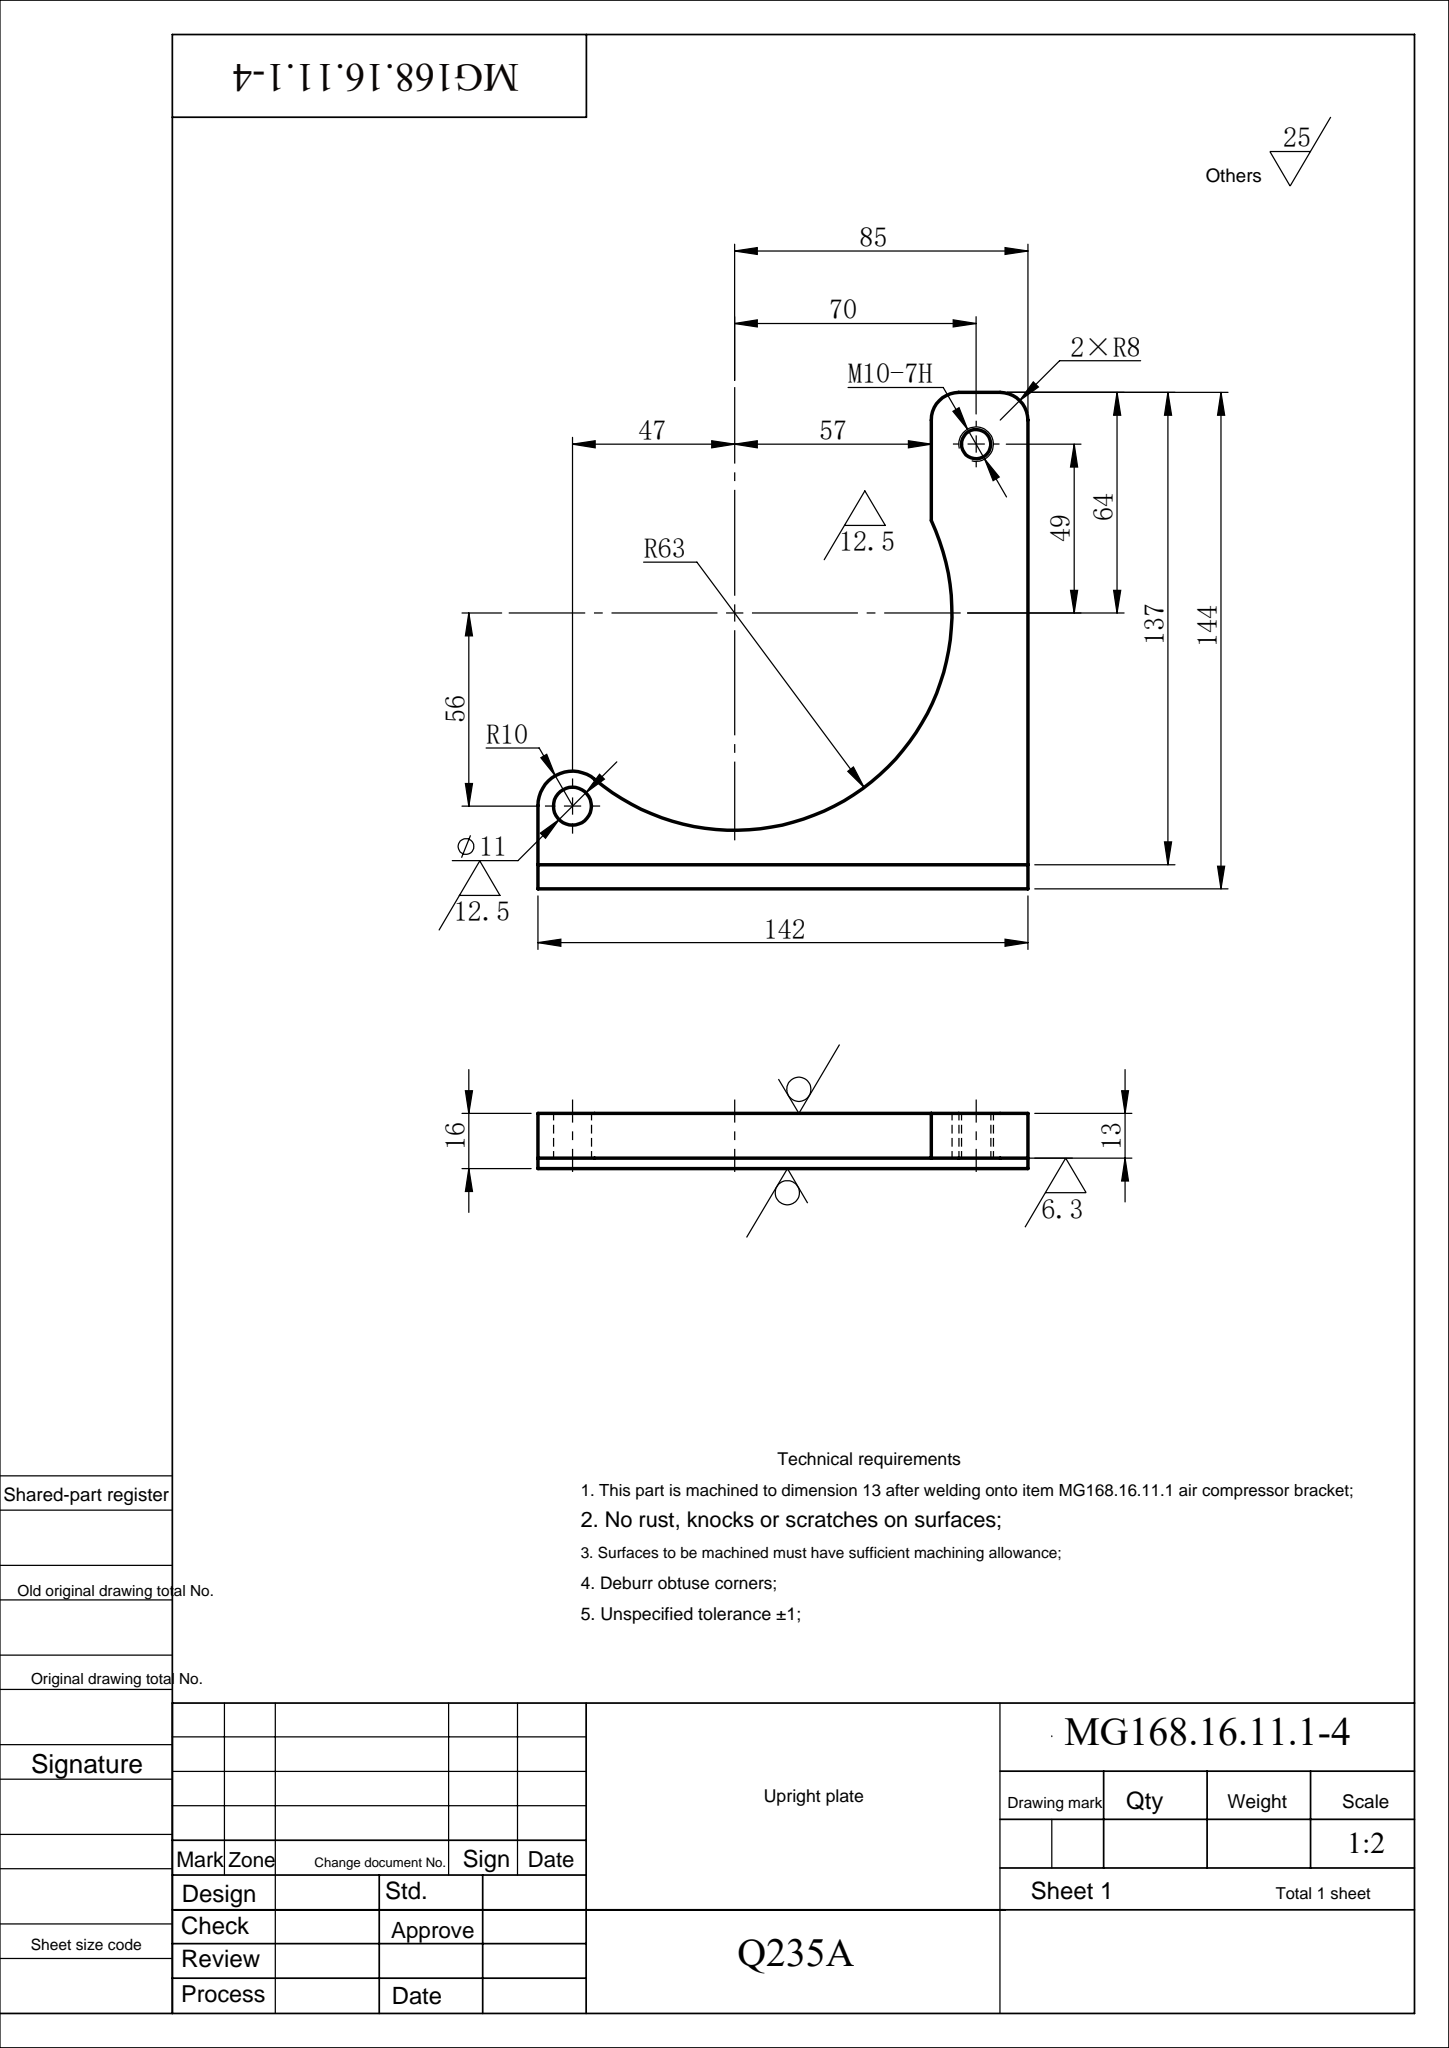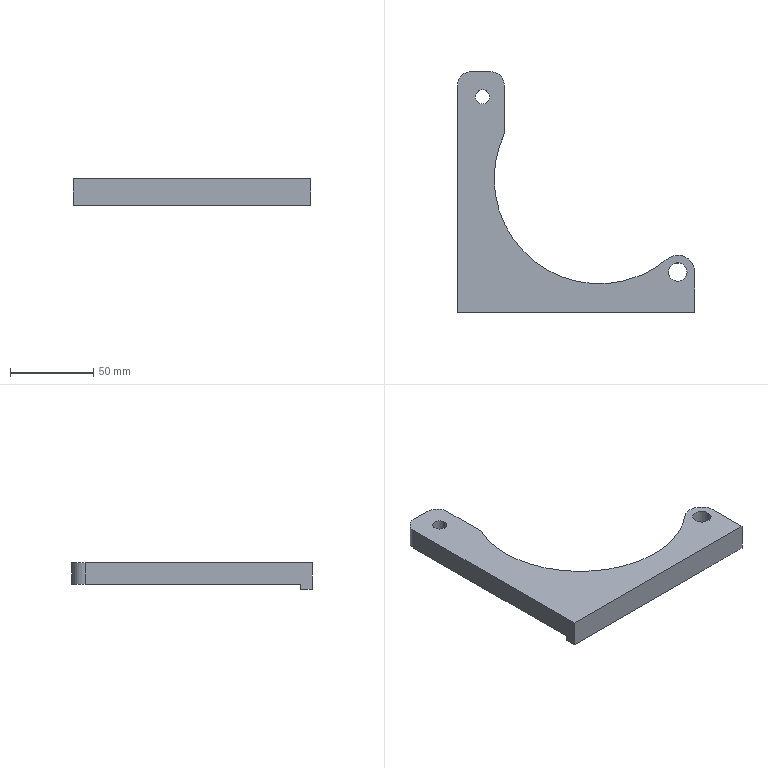Part | SolidWorks | features Extrusion 1, Fillet 1, HoleWzd 1, ICE 1 | 1 solid | 18 faces | box 142 x 144 x 16 mm | volume 88798 mm3 | cylinder 9 | plane 9 | commonest cylinder face diameters 8.5 x2 11 x2 16 x2 126 x2 20 x1
STEP:
#1=CARTESIAN_POINT('',(10.75,129.,-6.5));
#2=VERTEX_POINT('',#1);
#3=CARTESIAN_POINT('',(19.25,129.,-6.5));
#4=VERTEX_POINT('',#3);
#5=CARTESIAN_POINT('',(15.,129.,-6.5));
#6=DIRECTION('',(0.,0.,1.));
#7=DIRECTION('',(1.,0.,0.));
#8=AXIS2_PLACEMENT_3D('',#5,#6,#7);
#9=CIRCLE('',#8,4.25);
#10=EDGE_CURVE('',#2,#4,#9,.T.);
#11=ORIENTED_EDGE('',*,*,#10,.F.);
#12=CARTESIAN_POINT('',(10.75,129.,6.5));
#13=VERTEX_POINT('',#12);
#14=CARTESIAN_POINT('',(10.75,129.,6.5));
#15=DIRECTION('',(0.,0.,1.));
#16=VECTOR('',#15,1000.);
#17=LINE('',#14,#16);
#18=EDGE_CURVE('',#2,#13,#17,.T.);
#19=ORIENTED_EDGE('',*,*,#18,.T.);
#20=CARTESIAN_POINT('',(19.25,129.,6.5));
#21=VERTEX_POINT('',#20);
#22=CARTESIAN_POINT('',(15.,129.,6.5));
#23=DIRECTION('',(0.,0.,1.));
#24=DIRECTION('',(1.,0.,0.));
#25=AXIS2_PLACEMENT_3D('',#22,#23,#24);
#26=CIRCLE('',#25,4.25);
#27=EDGE_CURVE('',#13,#21,#26,.T.);
#28=ORIENTED_EDGE('',*,*,#27,.T.);
#29=CARTESIAN_POINT('',(19.25,129.,6.5));
#30=DIRECTION('',(0.,0.,1.));
#31=VECTOR('',#30,1000.);
#32=LINE('',#29,#31);
#33=EDGE_CURVE('',#4,#21,#32,.T.);
#34=ORIENTED_EDGE('',*,*,#33,.F.);
#35=EDGE_LOOP('',(#11,#19,#28,#34));
#36=FACE_OUTER_BOUND('',#35,.T.);
#37=CARTESIAN_POINT('',(15.,129.,6.5));
#38=DIRECTION('',(0.,0.,1.));
#39=DIRECTION('',(1.,0.,0.));
#40=AXIS2_PLACEMENT_3D('',#37,#38,#39);
#41=CYLINDRICAL_SURFACE('',#40,4.25);
#42=ADVANCED_FACE('',(#36),#41,.F.);
#43=CARTESIAN_POINT('',(126.5,24.,6.5));
#44=VERTEX_POINT('',#43);
#45=CARTESIAN_POINT('',(137.5,24.,6.5));
#46=VERTEX_POINT('',#45);
#47=CARTESIAN_POINT('',(132.,24.,6.5));
#48=DIRECTION('',(0.,0.,1.));
#49=DIRECTION('',(1.,0.,0.));
#50=AXIS2_PLACEMENT_3D('',#47,#48,#49);
#51=CIRCLE('',#50,5.5);
#52=EDGE_CURVE('',#44,#46,#51,.T.);
#53=ORIENTED_EDGE('',*,*,#52,.T.);
#54=CARTESIAN_POINT('',(137.5,24.,-6.5));
#55=VERTEX_POINT('',#54);
#56=CARTESIAN_POINT('',(137.5,24.,6.5));
#57=DIRECTION('',(0.,0.,-1.));
#58=VECTOR('',#57,1000.);
#59=LINE('',#56,#58);
#60=EDGE_CURVE('',#46,#55,#59,.T.);
#61=ORIENTED_EDGE('',*,*,#60,.T.);
#62=CARTESIAN_POINT('',(126.5,24.,-6.5));
#63=VERTEX_POINT('',#62);
#64=CARTESIAN_POINT('',(132.,24.,-6.5));
#65=DIRECTION('',(0.,0.,1.));
#66=DIRECTION('',(1.,0.,0.));
#67=AXIS2_PLACEMENT_3D('',#64,#65,#66);
#68=CIRCLE('',#67,5.5);
#69=EDGE_CURVE('',#63,#55,#68,.T.);
#70=ORIENTED_EDGE('',*,*,#69,.F.);
#71=CARTESIAN_POINT('',(126.5,24.,6.5));
#72=DIRECTION('',(0.,0.,-1.));
#73=VECTOR('',#72,1000.);
#74=LINE('',#71,#73);
#75=EDGE_CURVE('',#44,#63,#74,.T.);
#76=ORIENTED_EDGE('',*,*,#75,.F.);
#77=EDGE_LOOP('',(#53,#61,#70,#76));
#78=FACE_OUTER_BOUND('',#77,.T.);
#79=CARTESIAN_POINT('',(132.,24.,6.5));
#80=DIRECTION('',(0.,0.,-1.));
#81=DIRECTION('',(-1.,0.,0.));
#82=AXIS2_PLACEMENT_3D('',#79,#80,#81);
#83=CYLINDRICAL_SURFACE('',#82,5.5);
#84=ADVANCED_FACE('',(#78),#83,.F.);
#85=CARTESIAN_POINT('',(22.,80.,6.5));
#86=VERTEX_POINT('',#85);
#87=CARTESIAN_POINT('',(28.,106.833,6.5));
#88=VERTEX_POINT('',#87);
#89=CARTESIAN_POINT('',(85.,80.,6.5));
#90=DIRECTION('',(0.,0.,-1.));
#91=DIRECTION('',(1.,0.,0.));
#92=AXIS2_PLACEMENT_3D('',#89,#90,#91);
#93=CIRCLE('',#92,63.);
#94=EDGE_CURVE('',#86,#88,#93,.T.);
#95=ORIENTED_EDGE('',*,*,#94,.F.);
#96=CARTESIAN_POINT('',(22.,80.,-6.5));
#97=VERTEX_POINT('',#96);
#98=CARTESIAN_POINT('',(22.,80.,6.5));
#99=DIRECTION('',(0.,0.,-1.));
#100=VECTOR('',#99,1000.);
#101=LINE('',#98,#100);
#102=EDGE_CURVE('',#86,#97,#101,.T.);
#103=ORIENTED_EDGE('',*,*,#102,.T.);
#104=CARTESIAN_POINT('',(28.,106.833,-6.5));
#105=VERTEX_POINT('',#104);
#106=CARTESIAN_POINT('',(85.,80.,-6.5));
#107=DIRECTION('',(0.,0.,-1.));
#108=DIRECTION('',(1.,0.,0.));
#109=AXIS2_PLACEMENT_3D('',#106,#107,#108);
#110=CIRCLE('',#109,63.);
#111=EDGE_CURVE('',#97,#105,#110,.T.);
#112=ORIENTED_EDGE('',*,*,#111,.T.);
#113=CARTESIAN_POINT('',(28.,106.833,6.5));
#114=DIRECTION('',(0.,0.,-1.));
#115=VECTOR('',#114,1000.);
#116=LINE('',#113,#115);
#117=EDGE_CURVE('',#88,#105,#116,.T.);
#118=ORIENTED_EDGE('',*,*,#117,.F.);
#119=EDGE_LOOP('',(#95,#103,#112,#118));
#120=FACE_OUTER_BOUND('',#119,.T.);
#121=CARTESIAN_POINT('',(85.,80.,6.5));
#122=DIRECTION('',(0.,0.,-1.));
#123=DIRECTION('',(-1.,0.,0.));
#124=AXIS2_PLACEMENT_3D('',#121,#122,#123);
#125=CYLINDRICAL_SURFACE('',#124,63.);
#126=ADVANCED_FACE('',(#120),#125,.F.);
#127=CARTESIAN_POINT('',(15.,129.,6.5));
#128=DIRECTION('',(0.,0.,1.));
#129=DIRECTION('',(1.,0.,0.));
#130=AXIS2_PLACEMENT_3D('',#127,#128,#129);
#131=CIRCLE('',#130,4.25);
#132=EDGE_CURVE('',#21,#13,#131,.T.);
#133=ORIENTED_EDGE('',*,*,#132,.F.);
#134=ORIENTED_EDGE('',*,*,#27,.F.);
#135=EDGE_LOOP('',(#133,#134));
#136=FACE_BOUND('',#135,.T.);
#137=CARTESIAN_POINT('',(20.,144.,6.5));
#138=VERTEX_POINT('',#137);
#139=CARTESIAN_POINT('',(8.,144.,6.5));
#140=VERTEX_POINT('',#139);
#141=CARTESIAN_POINT('',(0.,144.,6.5));
#142=DIRECTION('',(-1.,0.,0.));
#143=VECTOR('',#142,1000.);
#144=LINE('',#141,#143);
#145=EDGE_CURVE('',#138,#140,#144,.T.);
#146=ORIENTED_EDGE('',*,*,#145,.T.);
#147=CARTESIAN_POINT('',(0.,136.,6.5));
#148=VERTEX_POINT('',#147);
#149=CARTESIAN_POINT('',(8.,136.,6.5));
#150=DIRECTION('',(0.,0.,1.));
#151=DIRECTION('',(1.,0.,0.));
#152=AXIS2_PLACEMENT_3D('',#149,#150,#151);
#153=CIRCLE('',#152,8.);
#154=EDGE_CURVE('',#140,#148,#153,.T.);
#155=ORIENTED_EDGE('',*,*,#154,.T.);
#156=CARTESIAN_POINT('',(0.,0.,6.5));
#157=VERTEX_POINT('',#156);
#158=CARTESIAN_POINT('',(0.,0.,6.5));
#159=DIRECTION('',(0.,-1.,0.));
#160=VECTOR('',#159,1000.);
#161=LINE('',#158,#160);
#162=EDGE_CURVE('',#148,#157,#161,.T.);
#163=ORIENTED_EDGE('',*,*,#162,.T.);
#164=CARTESIAN_POINT('',(142.,0.,6.5));
#165=VERTEX_POINT('',#164);
#166=CARTESIAN_POINT('',(0.,0.,6.5));
#167=DIRECTION('',(1.,0.,0.));
#168=VECTOR('',#167,1000.);
#169=LINE('',#166,#168);
#170=EDGE_CURVE('',#157,#165,#169,.T.);
#171=ORIENTED_EDGE('',*,*,#170,.T.);
#172=CARTESIAN_POINT('',(142.,24.143,6.5));
#173=VERTEX_POINT('',#172);
#174=CARTESIAN_POINT('',(142.,0.,6.5));
#175=DIRECTION('',(0.,1.,0.));
#176=VECTOR('',#175,1000.);
#177=LINE('',#174,#176);
#178=EDGE_CURVE('',#165,#173,#177,.T.);
#179=ORIENTED_EDGE('',*,*,#178,.T.);
#180=CARTESIAN_POINT('',(125.562,31.795,6.5));
#181=VERTEX_POINT('',#180);
#182=CARTESIAN_POINT('',(132.,24.143,6.5));
#183=DIRECTION('',(0.,0.,1.));
#184=DIRECTION('',(1.,0.,0.));
#185=AXIS2_PLACEMENT_3D('',#182,#183,#184);
#186=CIRCLE('',#185,10.);
#187=EDGE_CURVE('',#173,#181,#186,.T.);
#188=ORIENTED_EDGE('',*,*,#187,.T.);
#189=CARTESIAN_POINT('',(85.,80.,6.5));
#190=DIRECTION('',(0.,0.,-1.));
#191=DIRECTION('',(1.,0.,0.));
#192=AXIS2_PLACEMENT_3D('',#189,#190,#191);
#193=CIRCLE('',#192,63.);
#194=EDGE_CURVE('',#181,#86,#193,.T.);
#195=ORIENTED_EDGE('',*,*,#194,.T.);
#196=ORIENTED_EDGE('',*,*,#94,.T.);
#197=CARTESIAN_POINT('',(28.,136.,6.5));
#198=VERTEX_POINT('',#197);
#199=CARTESIAN_POINT('',(28.,144.,6.5));
#200=DIRECTION('',(0.,1.,0.));
#201=VECTOR('',#200,1000.);
#202=LINE('',#199,#201);
#203=EDGE_CURVE('',#88,#198,#202,.T.);
#204=ORIENTED_EDGE('',*,*,#203,.T.);
#205=CARTESIAN_POINT('',(20.,136.,6.5));
#206=DIRECTION('',(0.,0.,1.));
#207=DIRECTION('',(1.,0.,0.));
#208=AXIS2_PLACEMENT_3D('',#205,#206,#207);
#209=CIRCLE('',#208,8.);
#210=EDGE_CURVE('',#198,#138,#209,.T.);
#211=ORIENTED_EDGE('',*,*,#210,.T.);
#212=EDGE_LOOP('',(#146,#155,#163,#171,#179,#188,#195,#196,#204,#211));
#213=FACE_OUTER_BOUND('',#212,.T.);
#214=ORIENTED_EDGE('',*,*,#52,.F.);
#215=CARTESIAN_POINT('',(132.,24.,6.5));
#216=DIRECTION('',(0.,0.,1.));
#217=DIRECTION('',(1.,0.,0.));
#218=AXIS2_PLACEMENT_3D('',#215,#216,#217);
#219=CIRCLE('',#218,5.5);
#220=EDGE_CURVE('',#46,#44,#219,.T.);
#221=ORIENTED_EDGE('',*,*,#220,.F.);
#222=EDGE_LOOP('',(#214,#221));
#223=FACE_BOUND('',#222,.T.);
#224=CARTESIAN_POINT('',(85.,80.,6.5));
#225=DIRECTION('',(0.,0.,1.));
#226=DIRECTION('',(1.,0.,0.));
#227=AXIS2_PLACEMENT_3D('',#224,#225,#226);
#228=PLANE('',#227);
#229=ADVANCED_FACE('',(#136,#213,#223),#228,.T.);
#230=CARTESIAN_POINT('',(15.,129.,-6.5));
#231=DIRECTION('',(0.,0.,1.));
#232=DIRECTION('',(1.,0.,0.));
#233=AXIS2_PLACEMENT_3D('',#230,#231,#232);
#234=CIRCLE('',#233,4.25);
#235=EDGE_CURVE('',#4,#2,#234,.T.);
#236=ORIENTED_EDGE('',*,*,#235,.T.);
#237=ORIENTED_EDGE('',*,*,#10,.T.);
#238=EDGE_LOOP('',(#236,#237));
#239=FACE_BOUND('',#238,.T.);
#240=CARTESIAN_POINT('',(0.,136.,-6.5));
#241=VERTEX_POINT('',#240);
#242=CARTESIAN_POINT('',(0.,7.,-6.5));
#243=VERTEX_POINT('',#242);
#244=CARTESIAN_POINT('',(0.,0.,-6.5));
#245=DIRECTION('',(0.,-1.,0.));
#246=VECTOR('',#245,1000.);
#247=LINE('',#244,#246);
#248=EDGE_CURVE('',#241,#243,#247,.T.);
#249=ORIENTED_EDGE('',*,*,#248,.F.);
#250=CARTESIAN_POINT('',(8.,144.,-6.5));
#251=VERTEX_POINT('',#250);
#252=CARTESIAN_POINT('',(8.,136.,-6.5));
#253=DIRECTION('',(0.,0.,-1.));
#254=DIRECTION('',(1.,0.,0.));
#255=AXIS2_PLACEMENT_3D('',#252,#253,#254);
#256=CIRCLE('',#255,8.);
#257=EDGE_CURVE('',#241,#251,#256,.T.);
#258=ORIENTED_EDGE('',*,*,#257,.T.);
#259=CARTESIAN_POINT('',(20.,144.,-6.5));
#260=VERTEX_POINT('',#259);
#261=CARTESIAN_POINT('',(0.,144.,-6.5));
#262=DIRECTION('',(-1.,0.,0.));
#263=VECTOR('',#262,1000.);
#264=LINE('',#261,#263);
#265=EDGE_CURVE('',#260,#251,#264,.T.);
#266=ORIENTED_EDGE('',*,*,#265,.F.);
#267=CARTESIAN_POINT('',(28.,136.,-6.5));
#268=VERTEX_POINT('',#267);
#269=CARTESIAN_POINT('',(20.,136.,-6.5));
#270=DIRECTION('',(0.,0.,-1.));
#271=DIRECTION('',(1.,0.,0.));
#272=AXIS2_PLACEMENT_3D('',#269,#270,#271);
#273=CIRCLE('',#272,8.);
#274=EDGE_CURVE('',#260,#268,#273,.T.);
#275=ORIENTED_EDGE('',*,*,#274,.T.);
#276=CARTESIAN_POINT('',(28.,144.,-6.5));
#277=DIRECTION('',(0.,1.,0.));
#278=VECTOR('',#277,1000.);
#279=LINE('',#276,#278);
#280=EDGE_CURVE('',#105,#268,#279,.T.);
#281=ORIENTED_EDGE('',*,*,#280,.F.);
#282=ORIENTED_EDGE('',*,*,#111,.F.);
#283=CARTESIAN_POINT('',(125.562,31.795,-6.5));
#284=VERTEX_POINT('',#283);
#285=CARTESIAN_POINT('',(85.,80.,-6.5));
#286=DIRECTION('',(0.,0.,-1.));
#287=DIRECTION('',(1.,0.,0.));
#288=AXIS2_PLACEMENT_3D('',#285,#286,#287);
#289=CIRCLE('',#288,63.);
#290=EDGE_CURVE('',#284,#97,#289,.T.);
#291=ORIENTED_EDGE('',*,*,#290,.F.);
#292=CARTESIAN_POINT('',(142.,24.143,-6.5));
#293=VERTEX_POINT('',#292);
#294=CARTESIAN_POINT('',(132.,24.143,-6.5));
#295=DIRECTION('',(0.,0.,1.));
#296=DIRECTION('',(1.,0.,0.));
#297=AXIS2_PLACEMENT_3D('',#294,#295,#296);
#298=CIRCLE('',#297,10.);
#299=EDGE_CURVE('',#293,#284,#298,.T.);
#300=ORIENTED_EDGE('',*,*,#299,.F.);
#301=CARTESIAN_POINT('',(142.,7.,-6.5));
#302=VERTEX_POINT('',#301);
#303=CARTESIAN_POINT('',(142.,0.,-6.5));
#304=DIRECTION('',(0.,1.,0.));
#305=VECTOR('',#304,1000.);
#306=LINE('',#303,#305);
#307=EDGE_CURVE('',#302,#293,#306,.T.);
#308=ORIENTED_EDGE('',*,*,#307,.F.);
#309=CARTESIAN_POINT('',(0.,7.,-6.5));
#310=DIRECTION('',(-1.,0.,0.));
#311=VECTOR('',#310,1000.);
#312=LINE('',#309,#311);
#313=EDGE_CURVE('',#302,#243,#312,.T.);
#314=ORIENTED_EDGE('',*,*,#313,.T.);
#315=EDGE_LOOP('',(#249,#258,#266,#275,#281,#282,#291,#300,#308,#314));
#316=FACE_OUTER_BOUND('',#315,.T.);
#317=ORIENTED_EDGE('',*,*,#69,.T.);
#318=CARTESIAN_POINT('',(132.,24.,-6.5));
#319=DIRECTION('',(0.,0.,1.));
#320=DIRECTION('',(1.,0.,0.));
#321=AXIS2_PLACEMENT_3D('',#318,#319,#320);
#322=CIRCLE('',#321,5.5);
#323=EDGE_CURVE('',#55,#63,#322,.T.);
#324=ORIENTED_EDGE('',*,*,#323,.T.);
#325=EDGE_LOOP('',(#317,#324));
#326=FACE_BOUND('',#325,.T.);
#327=CARTESIAN_POINT('',(85.,80.,-6.5));
#328=DIRECTION('',(0.,0.,1.));
#329=DIRECTION('',(1.,0.,0.));
#330=AXIS2_PLACEMENT_3D('',#327,#328,#329);
#331=PLANE('',#330);
#332=ADVANCED_FACE('',(#239,#316,#326),#331,.F.);
#333=ORIENTED_EDGE('',*,*,#162,.F.);
#334=CARTESIAN_POINT('',(0.,136.,6.5));
#335=DIRECTION('',(0.,0.,-1.));
#336=VECTOR('',#335,1000.);
#337=LINE('',#334,#336);
#338=EDGE_CURVE('',#148,#241,#337,.T.);
#339=ORIENTED_EDGE('',*,*,#338,.T.);
#340=ORIENTED_EDGE('',*,*,#248,.T.);
#341=CARTESIAN_POINT('',(0.,7.,-9.5));
#342=VERTEX_POINT('',#341);
#343=CARTESIAN_POINT('',(0.,7.,-9.5));
#344=DIRECTION('',(0.,0.,1.));
#345=VECTOR('',#344,1000.);
#346=LINE('',#343,#345);
#347=EDGE_CURVE('',#342,#243,#346,.T.);
#348=ORIENTED_EDGE('',*,*,#347,.F.);
#349=CARTESIAN_POINT('',(0.,0.,-9.5));
#350=VERTEX_POINT('',#349);
#351=CARTESIAN_POINT('',(0.,0.,-9.5));
#352=DIRECTION('',(0.,-1.,0.));
#353=VECTOR('',#352,1000.);
#354=LINE('',#351,#353);
#355=EDGE_CURVE('',#342,#350,#354,.T.);
#356=ORIENTED_EDGE('',*,*,#355,.T.);
#357=CARTESIAN_POINT('',(0.,0.,6.5));
#358=DIRECTION('',(0.,0.,-1.));
#359=VECTOR('',#358,1000.);
#360=LINE('',#357,#359);
#361=EDGE_CURVE('',#157,#350,#360,.T.);
#362=ORIENTED_EDGE('',*,*,#361,.F.);
#363=EDGE_LOOP('',(#333,#339,#340,#348,#356,#362));
#364=FACE_OUTER_BOUND('',#363,.T.);
#365=CARTESIAN_POINT('',(0.,0.,6.5));
#366=DIRECTION('',(1.,0.,0.));
#367=DIRECTION('',(0.,0.,-1.));
#368=AXIS2_PLACEMENT_3D('',#365,#366,#367);
#369=PLANE('',#368);
#370=ADVANCED_FACE('',(#364),#369,.F.);
#371=ORIENTED_EDGE('',*,*,#361,.T.);
#372=CARTESIAN_POINT('',(142.,0.,-9.5));
#373=VERTEX_POINT('',#372);
#374=CARTESIAN_POINT('',(0.,0.,-9.5));
#375=DIRECTION('',(1.,0.,0.));
#376=VECTOR('',#375,1000.);
#377=LINE('',#374,#376);
#378=EDGE_CURVE('',#350,#373,#377,.T.);
#379=ORIENTED_EDGE('',*,*,#378,.T.);
#380=CARTESIAN_POINT('',(142.,0.,6.5));
#381=DIRECTION('',(0.,0.,-1.));
#382=VECTOR('',#381,1000.);
#383=LINE('',#380,#382);
#384=EDGE_CURVE('',#165,#373,#383,.T.);
#385=ORIENTED_EDGE('',*,*,#384,.F.);
#386=ORIENTED_EDGE('',*,*,#170,.F.);
#387=EDGE_LOOP('',(#371,#379,#385,#386));
#388=FACE_OUTER_BOUND('',#387,.T.);
#389=CARTESIAN_POINT('',(0.,0.,6.5));
#390=DIRECTION('',(0.,1.,0.));
#391=DIRECTION('',(0.,0.,1.));
#392=AXIS2_PLACEMENT_3D('',#389,#390,#391);
#393=PLANE('',#392);
#394=ADVANCED_FACE('',(#388),#393,.F.);
#395=ORIENTED_EDGE('',*,*,#384,.T.);
#396=CARTESIAN_POINT('',(142.,7.,-9.5));
#397=VERTEX_POINT('',#396);
#398=CARTESIAN_POINT('',(142.,0.,-9.5));
#399=DIRECTION('',(0.,1.,0.));
#400=VECTOR('',#399,1000.);
#401=LINE('',#398,#400);
#402=EDGE_CURVE('',#373,#397,#401,.T.);
#403=ORIENTED_EDGE('',*,*,#402,.T.);
#404=CARTESIAN_POINT('',(142.,7.,-9.5));
#405=DIRECTION('',(0.,0.,1.));
#406=VECTOR('',#405,1000.);
#407=LINE('',#404,#406);
#408=EDGE_CURVE('',#397,#302,#407,.T.);
#409=ORIENTED_EDGE('',*,*,#408,.T.);
#410=ORIENTED_EDGE('',*,*,#307,.T.);
#411=CARTESIAN_POINT('',(142.,24.143,6.5));
#412=DIRECTION('',(0.,0.,-1.));
#413=VECTOR('',#412,1000.);
#414=LINE('',#411,#413);
#415=EDGE_CURVE('',#173,#293,#414,.T.);
#416=ORIENTED_EDGE('',*,*,#415,.F.);
#417=ORIENTED_EDGE('',*,*,#178,.F.);
#418=EDGE_LOOP('',(#395,#403,#409,#410,#416,#417));
#419=FACE_OUTER_BOUND('',#418,.T.);
#420=CARTESIAN_POINT('',(142.,0.,6.5));
#421=DIRECTION('',(-1.,0.,0.));
#422=DIRECTION('',(0.,0.,1.));
#423=AXIS2_PLACEMENT_3D('',#420,#421,#422);
#424=PLANE('',#423);
#425=ADVANCED_FACE('',(#419),#424,.F.);
#426=ORIENTED_EDGE('',*,*,#299,.T.);
#427=CARTESIAN_POINT('',(125.562,31.795,6.5));
#428=DIRECTION('',(0.,0.,-1.));
#429=VECTOR('',#428,1000.);
#430=LINE('',#427,#429);
#431=EDGE_CURVE('',#181,#284,#430,.T.);
#432=ORIENTED_EDGE('',*,*,#431,.F.);
#433=ORIENTED_EDGE('',*,*,#187,.F.);
#434=ORIENTED_EDGE('',*,*,#415,.T.);
#435=EDGE_LOOP('',(#426,#432,#433,#434));
#436=FACE_OUTER_BOUND('',#435,.T.);
#437=CARTESIAN_POINT('',(132.,24.143,6.5));
#438=DIRECTION('',(0.,0.,-1.));
#439=DIRECTION('',(-1.,0.,0.));
#440=AXIS2_PLACEMENT_3D('',#437,#438,#439);
#441=CYLINDRICAL_SURFACE('',#440,10.);
#442=ADVANCED_FACE('',(#436),#441,.T.);
#443=ORIENTED_EDGE('',*,*,#102,.F.);
#444=ORIENTED_EDGE('',*,*,#194,.F.);
#445=ORIENTED_EDGE('',*,*,#431,.T.);
#446=ORIENTED_EDGE('',*,*,#290,.T.);
#447=EDGE_LOOP('',(#443,#444,#445,#446));
#448=FACE_OUTER_BOUND('',#447,.T.);
#449=CARTESIAN_POINT('',(85.,80.,6.5));
#450=DIRECTION('',(0.,0.,-1.));
#451=DIRECTION('',(-1.,0.,0.));
#452=AXIS2_PLACEMENT_3D('',#449,#450,#451);
#453=CYLINDRICAL_SURFACE('',#452,63.);
#454=ADVANCED_FACE('',(#448),#453,.F.);
#455=ORIENTED_EDGE('',*,*,#280,.T.);
#456=CARTESIAN_POINT('',(28.,136.,6.5));
#457=DIRECTION('',(0.,0.,1.));
#458=VECTOR('',#457,1000.);
#459=LINE('',#456,#458);
#460=EDGE_CURVE('',#268,#198,#459,.T.);
#461=ORIENTED_EDGE('',*,*,#460,.T.);
#462=ORIENTED_EDGE('',*,*,#203,.F.);
#463=ORIENTED_EDGE('',*,*,#117,.T.);
#464=EDGE_LOOP('',(#455,#461,#462,#463));
#465=FACE_OUTER_BOUND('',#464,.T.);
#466=CARTESIAN_POINT('',(28.,144.,6.5));
#467=DIRECTION('',(-1.,0.,0.));
#468=DIRECTION('',(0.,-1.,0.));
#469=AXIS2_PLACEMENT_3D('',#466,#467,#468);
#470=PLANE('',#469);
#471=ADVANCED_FACE('',(#465),#470,.F.);
#472=ORIENTED_EDGE('',*,*,#265,.T.);
#473=CARTESIAN_POINT('',(8.,144.,6.5));
#474=DIRECTION('',(0.,0.,1.));
#475=VECTOR('',#474,1000.);
#476=LINE('',#473,#475);
#477=EDGE_CURVE('',#251,#140,#476,.T.);
#478=ORIENTED_EDGE('',*,*,#477,.T.);
#479=ORIENTED_EDGE('',*,*,#145,.F.);
#480=CARTESIAN_POINT('',(20.,144.,6.5));
#481=DIRECTION('',(0.,0.,-1.));
#482=VECTOR('',#481,1000.);
#483=LINE('',#480,#482);
#484=EDGE_CURVE('',#138,#260,#483,.T.);
#485=ORIENTED_EDGE('',*,*,#484,.T.);
#486=EDGE_LOOP('',(#472,#478,#479,#485));
#487=FACE_OUTER_BOUND('',#486,.T.);
#488=CARTESIAN_POINT('',(0.,144.,6.5));
#489=DIRECTION('',(0.,-1.,0.));
#490=DIRECTION('',(0.,0.,-1.));
#491=AXIS2_PLACEMENT_3D('',#488,#489,#490);
#492=PLANE('',#491);
#493=ADVANCED_FACE('',(#487),#492,.F.);
#494=ORIENTED_EDGE('',*,*,#60,.F.);
#495=ORIENTED_EDGE('',*,*,#220,.T.);
#496=ORIENTED_EDGE('',*,*,#75,.T.);
#497=ORIENTED_EDGE('',*,*,#323,.F.);
#498=EDGE_LOOP('',(#494,#495,#496,#497));
#499=FACE_OUTER_BOUND('',#498,.T.);
#500=CARTESIAN_POINT('',(132.,24.,6.5));
#501=DIRECTION('',(0.,0.,-1.));
#502=DIRECTION('',(-1.,0.,0.));
#503=AXIS2_PLACEMENT_3D('',#500,#501,#502);
#504=CYLINDRICAL_SURFACE('',#503,5.5);
#505=ADVANCED_FACE('',(#499),#504,.F.);
#506=ORIENTED_EDGE('',*,*,#313,.F.);
#507=ORIENTED_EDGE('',*,*,#408,.F.);
#508=CARTESIAN_POINT('',(0.,7.,-9.5));
#509=DIRECTION('',(-1.,0.,0.));
#510=VECTOR('',#509,1000.);
#511=LINE('',#508,#510);
#512=EDGE_CURVE('',#397,#342,#511,.T.);
#513=ORIENTED_EDGE('',*,*,#512,.T.);
#514=ORIENTED_EDGE('',*,*,#347,.T.);
#515=EDGE_LOOP('',(#506,#507,#513,#514));
#516=FACE_OUTER_BOUND('',#515,.T.);
#517=CARTESIAN_POINT('',(0.,7.,-9.5));
#518=DIRECTION('',(0.,1.,0.));
#519=DIRECTION('',(0.,0.,1.));
#520=AXIS2_PLACEMENT_3D('',#517,#518,#519);
#521=PLANE('',#520);
#522=ADVANCED_FACE('',(#516),#521,.T.);
#523=ORIENTED_EDGE('',*,*,#355,.F.);
#524=ORIENTED_EDGE('',*,*,#512,.F.);
#525=ORIENTED_EDGE('',*,*,#402,.F.);
#526=ORIENTED_EDGE('',*,*,#378,.F.);
#527=EDGE_LOOP('',(#523,#524,#525,#526));
#528=FACE_OUTER_BOUND('',#527,.T.);
#529=CARTESIAN_POINT('',(0.,0.,-9.5));
#530=DIRECTION('',(0.,0.,-1.));
#531=DIRECTION('',(-1.,0.,0.));
#532=AXIS2_PLACEMENT_3D('',#529,#530,#531);
#533=PLANE('',#532);
#534=ADVANCED_FACE('',(#528),#533,.T.);
#535=ORIENTED_EDGE('',*,*,#18,.F.);
#536=ORIENTED_EDGE('',*,*,#235,.F.);
#537=ORIENTED_EDGE('',*,*,#33,.T.);
#538=ORIENTED_EDGE('',*,*,#132,.T.);
#539=EDGE_LOOP('',(#535,#536,#537,#538));
#540=FACE_OUTER_BOUND('',#539,.T.);
#541=CARTESIAN_POINT('',(15.,129.,6.5));
#542=DIRECTION('',(0.,0.,1.));
#543=DIRECTION('',(1.,0.,0.));
#544=AXIS2_PLACEMENT_3D('',#541,#542,#543);
#545=CYLINDRICAL_SURFACE('',#544,4.25);
#546=ADVANCED_FACE('',(#540),#545,.F.);
#547=ORIENTED_EDGE('',*,*,#154,.F.);
#548=ORIENTED_EDGE('',*,*,#477,.F.);
#549=ORIENTED_EDGE('',*,*,#257,.F.);
#550=ORIENTED_EDGE('',*,*,#338,.F.);
#551=EDGE_LOOP('',(#547,#548,#549,#550));
#552=FACE_OUTER_BOUND('',#551,.T.);
#553=CARTESIAN_POINT('',(8.,136.,6.5));
#554=DIRECTION('',(0.,0.,-1.));
#555=DIRECTION('',(-1.,0.,0.));
#556=AXIS2_PLACEMENT_3D('',#553,#554,#555);
#557=CYLINDRICAL_SURFACE('',#556,8.);
#558=ADVANCED_FACE('',(#552),#557,.T.);
#559=ORIENTED_EDGE('',*,*,#210,.F.);
#560=ORIENTED_EDGE('',*,*,#460,.F.);
#561=ORIENTED_EDGE('',*,*,#274,.F.);
#562=ORIENTED_EDGE('',*,*,#484,.F.);
#563=EDGE_LOOP('',(#559,#560,#561,#562));
#564=FACE_OUTER_BOUND('',#563,.T.);
#565=CARTESIAN_POINT('',(20.,136.,6.5));
#566=DIRECTION('',(0.,0.,-1.));
#567=DIRECTION('',(-1.,0.,0.));
#568=AXIS2_PLACEMENT_3D('',#565,#566,#567);
#569=CYLINDRICAL_SURFACE('',#568,8.);
#570=ADVANCED_FACE('',(#564),#569,.T.);
#571=CLOSED_SHELL('',(#42,#84,#126,#229,#332,#370,#394,#425,#442,#454,#471,#493,#505,#522,#534,#546,#558,#570));
#572=MANIFOLD_SOLID_BREP('',#571);
#573=CARTESIAN_POINT('',(0.,0.,0.));
#574=DIRECTION('',(0.,0.,1.));
#575=DIRECTION('',(1.,0.,0.));
#576=AXIS2_PLACEMENT_3D('',#573,#574,#575);
#577=(LENGTH_UNIT()NAMED_UNIT(*)SI_UNIT(.MILLI.,.METRE.));
#578=UNCERTAINTY_MEASURE_WITH_UNIT(LENGTH_MEASURE(0.00001),#577,'','');
#579=(NAMED_UNIT(*)PLANE_ANGLE_UNIT()SI_UNIT($,.RADIAN.));
#580=(NAMED_UNIT(*)SI_UNIT($,.STERADIAN.)SOLID_ANGLE_UNIT());
#581=(GEOMETRIC_REPRESENTATION_CONTEXT(3)GLOBAL_UNCERTAINTY_ASSIGNED_CONTEXT((#578))GLOBAL_UNIT_ASSIGNED_CONTEXT((#577,#579,#580))REPRESENTATION_CONTEXT('',''));
#582=ADVANCED_BREP_SHAPE_REPRESENTATION('',(#572,#576),#581);